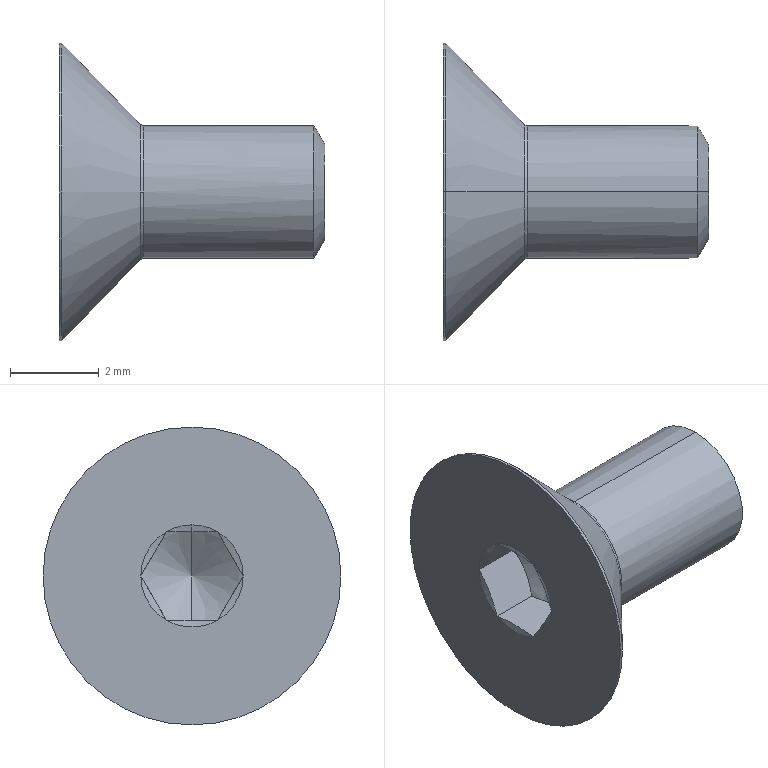Part | SolidWorks | features BaseBody 1 | 1 solid | 27 faces | box 6 x 6.72 x 6.72 mm | volume 61.288 mm3 | cone 13 | plane 8 | cylinder 4 | spline 2 | commonest cylinder face diameters 3 x2 6.72 x2
STEP:
#1=CARTESIAN_POINT('',(-4.169,-1.531,0.));
#2=VERTEX_POINT('',#1);
#3=CARTESIAN_POINT('',(-4.169,0.,1.531));
#4=VERTEX_POINT('',#3);
#5=CARTESIAN_POINT('',(-4.169,0.,0.));
#6=DIRECTION('',(-1.,0.,0.));
#7=DIRECTION('',(0.,-1.,0.));
#8=AXIS2_PLACEMENT_3D('',#5,#6,#7);
#9=CIRCLE('',#8,1.531);
#10=EDGE_CURVE('',#2,#4,#9,.T.);
#11=ORIENTED_EDGE('',*,*,#10,.F.);
#12=CARTESIAN_POINT('',(-4.098,-1.5,0.));
#13=VERTEX_POINT('',#12);
#14=CARTESIAN_POINT('',(-4.098,-1.6,0.));
#15=DIRECTION('',(0.,0.,-1.));
#16=DIRECTION('',(0.,-1.,0.));
#17=AXIS2_PLACEMENT_3D('',#14,#15,#16);
#18=CIRCLE('',#17,0.1);
#19=EDGE_CURVE('',#2,#13,#18,.T.);
#20=ORIENTED_EDGE('',*,*,#19,.T.);
#21=CARTESIAN_POINT('',(-4.098,0.,1.5));
#22=VERTEX_POINT('',#21);
#23=CARTESIAN_POINT('',(-4.098,0.,0.));
#24=DIRECTION('',(1.,0.,0.));
#25=DIRECTION('',(0.,1.,0.));
#26=AXIS2_PLACEMENT_3D('',#23,#24,#25);
#27=CIRCLE('',#26,1.5);
#28=EDGE_CURVE('',#22,#13,#27,.T.);
#29=ORIENTED_EDGE('',*,*,#28,.F.);
#30=CARTESIAN_POINT('',(-4.098,1.5,0.));
#31=VERTEX_POINT('',#30);
#32=CARTESIAN_POINT('',(-4.098,0.,0.));
#33=DIRECTION('',(1.,0.,0.));
#34=DIRECTION('',(0.,1.,0.));
#35=AXIS2_PLACEMENT_3D('',#32,#33,#34);
#36=CIRCLE('',#35,1.5);
#37=EDGE_CURVE('',#31,#22,#36,.T.);
#38=ORIENTED_EDGE('',*,*,#37,.F.);
#39=CARTESIAN_POINT('',(-4.169,1.531,0.));
#40=VERTEX_POINT('',#39);
#41=CARTESIAN_POINT('',(-4.098,1.6,0.));
#42=DIRECTION('',(0.,0.,1.));
#43=DIRECTION('',(0.,1.,0.));
#44=AXIS2_PLACEMENT_3D('',#41,#42,#43);
#45=CIRCLE('',#44,0.1);
#46=EDGE_CURVE('',#40,#31,#45,.T.);
#47=ORIENTED_EDGE('',*,*,#46,.F.);
#48=CARTESIAN_POINT('',(-4.169,0.,0.));
#49=DIRECTION('',(-1.,0.,0.));
#50=DIRECTION('',(0.,-1.,0.));
#51=AXIS2_PLACEMENT_3D('',#48,#49,#50);
#52=CIRCLE('',#51,1.531);
#53=EDGE_CURVE('',#4,#40,#52,.T.);
#54=ORIENTED_EDGE('',*,*,#53,.F.);
#55=EDGE_LOOP('',(#11,#20,#29,#38,#47,#54));
#56=FACE_OUTER_BOUND('',#55,.T.);
#57=CARTESIAN_POINT('',(-4.169,1.531,0.));
#58=CARTESIAN_POINT('',(-4.169,1.531,3.061));
#59=CARTESIAN_POINT('',(-4.169,-1.531,3.061));
#60=CARTESIAN_POINT('',(-4.169,-1.531,0.));
#61=CARTESIAN_POINT('',(-4.15,1.511,0.));
#62=CARTESIAN_POINT('',(-4.15,1.511,3.021));
#63=CARTESIAN_POINT('',(-4.15,-1.511,3.021));
#64=CARTESIAN_POINT('',(-4.15,-1.511,0.));
#65=CARTESIAN_POINT('',(-4.125,1.5,0.));
#66=CARTESIAN_POINT('',(-4.125,1.5,3.));
#67=CARTESIAN_POINT('',(-4.125,-1.5,3.));
#68=CARTESIAN_POINT('',(-4.125,-1.5,0.));
#69=CARTESIAN_POINT('',(-4.098,1.5,0.));
#70=CARTESIAN_POINT('',(-4.098,1.5,3.));
#71=CARTESIAN_POINT('',(-4.098,-1.5,3.));
#72=CARTESIAN_POINT('',(-4.098,-1.5,0.));
#73=(BOUNDED_SURFACE()B_SPLINE_SURFACE(3,3,((#57,#58,#59,#60),(#61,#62,#63,#64),(#65,#66,#67,#68),(#69,#70,#71,#72)),.UNSPECIFIED.,.F.,.F.,.F.)B_SPLINE_SURFACE_WITH_KNOTS((4,4),(4,4),(0.,1.),(0.,1.),.UNSPECIFIED.)GEOMETRIC_REPRESENTATION_ITEM()RATIONAL_B_SPLINE_SURFACE(((1.,0.3333,0.3333,1.),(0.947,0.3157,0.3157,0.947),(0.947,0.3157,0.3157,0.947),(1.,0.3333,0.3333,1.)))REPRESENTATION_ITEM('')SURFACE());
#74=ADVANCED_FACE('',(#56),#73,.F.);
#75=ORIENTED_EDGE('',*,*,#53,.T.);
#76=CARTESIAN_POINT('',(-4.169,0.,-1.531));
#77=VERTEX_POINT('',#76);
#78=CARTESIAN_POINT('',(-4.169,0.,0.));
#79=DIRECTION('',(-1.,0.,0.));
#80=DIRECTION('',(0.,-1.,0.));
#81=AXIS2_PLACEMENT_3D('',#78,#79,#80);
#82=CIRCLE('',#81,1.531);
#83=EDGE_CURVE('',#40,#77,#82,.T.);
#84=ORIENTED_EDGE('',*,*,#83,.T.);
#85=CARTESIAN_POINT('',(-5.936,0.,-3.36));
#86=VERTEX_POINT('',#85);
#87=CARTESIAN_POINT('',(-5.936,0.,-3.36));
#88=DIRECTION('',(-0.6947,0.,-0.7193));
#89=VECTOR('',#88,1000.);
#90=LINE('',#87,#89);
#91=EDGE_CURVE('',#77,#86,#90,.T.);
#92=ORIENTED_EDGE('',*,*,#91,.T.);
#93=CARTESIAN_POINT('',(-5.936,0.,3.36));
#94=VERTEX_POINT('',#93);
#95=CARTESIAN_POINT('',(-5.936,0.,0.));
#96=DIRECTION('',(1.,0.,0.));
#97=DIRECTION('',(0.,-1.,0.));
#98=AXIS2_PLACEMENT_3D('',#95,#96,#97);
#99=CIRCLE('',#98,3.36);
#100=EDGE_CURVE('',#86,#94,#99,.T.);
#101=ORIENTED_EDGE('',*,*,#100,.T.);
#102=CARTESIAN_POINT('',(-5.936,0.,3.36));
#103=DIRECTION('',(-0.6947,0.,0.7193));
#104=VECTOR('',#103,1000.);
#105=LINE('',#102,#104);
#106=EDGE_CURVE('',#4,#94,#105,.T.);
#107=ORIENTED_EDGE('',*,*,#106,.F.);
#108=EDGE_LOOP('',(#75,#84,#92,#101,#107));
#109=FACE_OUTER_BOUND('',#108,.T.);
#110=CARTESIAN_POINT('',(-5.936,0.,0.));
#111=DIRECTION('',(-1.,0.,0.));
#112=DIRECTION('',(0.,0.,1.));
#113=AXIS2_PLACEMENT_3D('',#110,#111,#112);
#114=CONICAL_SURFACE('',#113,3.36,0.8029);
#115=ADVANCED_FACE('',(#109),#114,.T.);
#116=CARTESIAN_POINT('',(-6.,0.,-3.36));
#117=VERTEX_POINT('',#116);
#118=CARTESIAN_POINT('',(-6.,0.,3.36));
#119=VERTEX_POINT('',#118);
#120=CARTESIAN_POINT('',(-6.,0.,0.));
#121=DIRECTION('',(1.,0.,0.));
#122=DIRECTION('',(0.,0.,-1.));
#123=AXIS2_PLACEMENT_3D('',#120,#121,#122);
#124=CIRCLE('',#123,3.36);
#125=EDGE_CURVE('',#117,#119,#124,.T.);
#126=ORIENTED_EDGE('',*,*,#125,.T.);
#127=CARTESIAN_POINT('',(0.,0.,3.36));
#128=DIRECTION('',(1.,0.,0.));
#129=VECTOR('',#128,1000.);
#130=LINE('',#127,#129);
#131=EDGE_CURVE('',#119,#94,#130,.T.);
#132=ORIENTED_EDGE('',*,*,#131,.T.);
#133=ORIENTED_EDGE('',*,*,#100,.F.);
#134=CARTESIAN_POINT('',(0.,0.,-3.36));
#135=DIRECTION('',(1.,0.,0.));
#136=VECTOR('',#135,1000.);
#137=LINE('',#134,#136);
#138=EDGE_CURVE('',#117,#86,#137,.T.);
#139=ORIENTED_EDGE('',*,*,#138,.F.);
#140=EDGE_LOOP('',(#126,#132,#133,#139));
#141=FACE_OUTER_BOUND('',#140,.T.);
#142=CARTESIAN_POINT('',(0.,0.,0.));
#143=DIRECTION('',(1.,0.,0.));
#144=DIRECTION('',(0.,0.,-1.));
#145=AXIS2_PLACEMENT_3D('',#142,#143,#144);
#146=CYLINDRICAL_SURFACE('',#145,3.36);
#147=ADVANCED_FACE('',(#141),#146,.T.);
#148=CARTESIAN_POINT('',(-4.098,0.,-1.5));
#149=VERTEX_POINT('',#148);
#150=CARTESIAN_POINT('',(-4.098,0.,0.));
#151=DIRECTION('',(1.,0.,0.));
#152=DIRECTION('',(0.,1.,0.));
#153=AXIS2_PLACEMENT_3D('',#150,#151,#152);
#154=CIRCLE('',#153,1.5);
#155=EDGE_CURVE('',#149,#31,#154,.T.);
#156=ORIENTED_EDGE('',*,*,#155,.T.);
#157=ORIENTED_EDGE('',*,*,#37,.T.);
#158=CARTESIAN_POINT('',(-0.25,0.,1.5));
#159=VERTEX_POINT('',#158);
#160=CARTESIAN_POINT('',(0.,0.,1.5));
#161=DIRECTION('',(1.,0.,0.));
#162=VECTOR('',#161,1000.);
#163=LINE('',#160,#162);
#164=EDGE_CURVE('',#22,#159,#163,.T.);
#165=ORIENTED_EDGE('',*,*,#164,.T.);
#166=CARTESIAN_POINT('',(-0.25,0.,-1.5));
#167=VERTEX_POINT('',#166);
#168=CARTESIAN_POINT('',(-0.25,0.,0.));
#169=DIRECTION('',(-1.,0.,0.));
#170=DIRECTION('',(0.,0.,-1.));
#171=AXIS2_PLACEMENT_3D('',#168,#169,#170);
#172=CIRCLE('',#171,1.5);
#173=EDGE_CURVE('',#159,#167,#172,.T.);
#174=ORIENTED_EDGE('',*,*,#173,.T.);
#175=CARTESIAN_POINT('',(0.,0.,-1.5));
#176=DIRECTION('',(1.,0.,0.));
#177=VECTOR('',#176,1000.);
#178=LINE('',#175,#177);
#179=EDGE_CURVE('',#149,#167,#178,.T.);
#180=ORIENTED_EDGE('',*,*,#179,.F.);
#181=EDGE_LOOP('',(#156,#157,#165,#174,#180));
#182=FACE_OUTER_BOUND('',#181,.T.);
#183=CARTESIAN_POINT('',(0.,0.,0.));
#184=DIRECTION('',(1.,0.,0.));
#185=DIRECTION('',(0.,0.,-1.));
#186=AXIS2_PLACEMENT_3D('',#183,#184,#185);
#187=CYLINDRICAL_SURFACE('',#186,1.5);
#188=ADVANCED_FACE('',(#182),#187,.T.);
#189=CARTESIAN_POINT('',(0.,0.,1.067));
#190=VERTEX_POINT('',#189);
#191=CARTESIAN_POINT('',(0.,0.,-1.067));
#192=VERTEX_POINT('',#191);
#193=CARTESIAN_POINT('',(0.,0.,0.));
#194=DIRECTION('',(-1.,0.,0.));
#195=DIRECTION('',(0.,0.,1.));
#196=AXIS2_PLACEMENT_3D('',#193,#194,#195);
#197=CIRCLE('',#196,1.067);
#198=EDGE_CURVE('',#190,#192,#197,.T.);
#199=ORIENTED_EDGE('',*,*,#198,.T.);
#200=CARTESIAN_POINT('',(-0.25,0.,-1.5));
#201=DIRECTION('',(-0.5,0.,-0.866));
#202=VECTOR('',#201,1000.);
#203=LINE('',#200,#202);
#204=EDGE_CURVE('',#192,#167,#203,.T.);
#205=ORIENTED_EDGE('',*,*,#204,.T.);
#206=ORIENTED_EDGE('',*,*,#173,.F.);
#207=CARTESIAN_POINT('',(-0.25,0.,1.5));
#208=DIRECTION('',(-0.5,0.,0.866));
#209=VECTOR('',#208,1000.);
#210=LINE('',#207,#209);
#211=EDGE_CURVE('',#190,#159,#210,.T.);
#212=ORIENTED_EDGE('',*,*,#211,.F.);
#213=EDGE_LOOP('',(#199,#205,#206,#212));
#214=FACE_OUTER_BOUND('',#213,.T.);
#215=CARTESIAN_POINT('',(-0.25,0.,0.));
#216=DIRECTION('',(-1.,0.,0.));
#217=DIRECTION('',(0.,0.,1.));
#218=AXIS2_PLACEMENT_3D('',#215,#216,#217);
#219=CONICAL_SURFACE('',#218,1.5,1.047);
#220=ADVANCED_FACE('',(#214),#219,.T.);
#221=CARTESIAN_POINT('',(-5.956,0.,1.));
#222=VERTEX_POINT('',#221);
#223=CARTESIAN_POINT('',(-6.,0.5774,1.));
#224=VERTEX_POINT('',#223);
#225=CARTESIAN_POINT('',(-5.956,0.,1.));
#226=CARTESIAN_POINT('',(-5.956,0.1925,1.));
#227=CARTESIAN_POINT('',(-5.973,0.3849,1.));
#228=CARTESIAN_POINT('',(-6.,0.5774,1.));
#229=B_SPLINE_CURVE_WITH_KNOTS('',3,(#225,#226,#227,#228),.UNSPECIFIED.,.F.,.F.,(4,4),(0.0005774,0.001155),.UNSPECIFIED.);
#230=EDGE_CURVE('',#222,#224,#229,.T.);
#231=ORIENTED_EDGE('',*,*,#230,.F.);
#232=CARTESIAN_POINT('',(-6.,0.,1.155));
#233=VERTEX_POINT('',#232);
#234=CARTESIAN_POINT('',(-6.,0.,1.155));
#235=DIRECTION('',(-0.2748,0.,0.9615));
#236=VECTOR('',#235,1000.);
#237=LINE('',#234,#236);
#238=EDGE_CURVE('',#222,#233,#237,.T.);
#239=ORIENTED_EDGE('',*,*,#238,.T.);
#240=CARTESIAN_POINT('',(-6.,0.,0.));
#241=DIRECTION('',(1.,0.,0.));
#242=DIRECTION('',(0.,0.,1.));
#243=AXIS2_PLACEMENT_3D('',#240,#241,#242);
#244=CIRCLE('',#243,1.155);
#245=EDGE_CURVE('',#224,#233,#244,.T.);
#246=ORIENTED_EDGE('',*,*,#245,.F.);
#247=EDGE_LOOP('',(#231,#239,#246));
#248=FACE_OUTER_BOUND('',#247,.T.);
#249=CARTESIAN_POINT('',(-6.,0.,0.));
#250=DIRECTION('',(-1.,0.,0.));
#251=DIRECTION('',(0.,0.,1.));
#252=AXIS2_PLACEMENT_3D('',#249,#250,#251);
#253=CONICAL_SURFACE('',#252,1.155,1.292);
#254=ADVANCED_FACE('',(#248),#253,.F.);
#255=CARTESIAN_POINT('',(-4.233,0.,0.));
#256=VERTEX_POINT('',#255);
#257=CARTESIAN_POINT('',(-4.811,0.,1.));
#258=VERTEX_POINT('',#257);
#259=CARTESIAN_POINT('',(-4.904,0.,1.162));
#260=DIRECTION('',(-0.5,0.,0.866));
#261=VECTOR('',#260,1000.);
#262=LINE('',#259,#261);
#263=EDGE_CURVE('',#256,#258,#262,.T.);
#264=ORIENTED_EDGE('',*,*,#263,.F.);
#265=CARTESIAN_POINT('',(-4.811,0.,-1.));
#266=VERTEX_POINT('',#265);
#267=CARTESIAN_POINT('',(-4.904,0.,-1.162));
#268=DIRECTION('',(-0.5,0.,-0.866));
#269=VECTOR('',#268,1000.);
#270=LINE('',#267,#269);
#271=EDGE_CURVE('',#256,#266,#270,.T.);
#272=ORIENTED_EDGE('',*,*,#271,.T.);
#273=CARTESIAN_POINT('',(-4.9,-0.5774,-1.));
#274=VERTEX_POINT('',#273);
#275=CARTESIAN_POINT('',(-4.811,0.,-1.));
#276=CARTESIAN_POINT('',(-4.811,-0.196,-1.));
#277=CARTESIAN_POINT('',(-4.846,-0.3889,-1.));
#278=CARTESIAN_POINT('',(-4.9,-0.5774,-1.));
#279=B_SPLINE_CURVE_WITH_KNOTS('',3,(#275,#276,#277,#278),.UNSPECIFIED.,.F.,.F.,(4,4),(0.0005842,0.001166),.UNSPECIFIED.);
#280=EDGE_CURVE('',#266,#274,#279,.T.);
#281=ORIENTED_EDGE('',*,*,#280,.T.);
#282=CARTESIAN_POINT('',(-4.9,-1.155,0.));
#283=VERTEX_POINT('',#282);
#284=CARTESIAN_POINT('',(-4.9,-0.5774,-1.));
#285=CARTESIAN_POINT('',(-4.846,-0.6716,-0.8367));
#286=CARTESIAN_POINT('',(-4.811,-0.7673,-0.671));
#287=CARTESIAN_POINT('',(-4.811,-0.9636,-0.3309));
#288=CARTESIAN_POINT('',(-4.846,-1.06,-0.1635));
#289=CARTESIAN_POINT('',(-4.9,-1.155,0.));
#290=B_SPLINE_CURVE_WITH_KNOTS('',3,(#284,#285,#286,#287,#288,#289),.UNSPECIFIED.,.F.,.F.,(4,2,4),(0.,0.0005831,0.001166),.UNSPECIFIED.);
#291=EDGE_CURVE('',#274,#283,#290,.T.);
#292=ORIENTED_EDGE('',*,*,#291,.T.);
#293=CARTESIAN_POINT('',(-4.9,-0.5774,1.));
#294=VERTEX_POINT('',#293);
#295=CARTESIAN_POINT('',(-4.9,-1.155,0.));
#296=CARTESIAN_POINT('',(-4.846,-1.06,0.1633));
#297=CARTESIAN_POINT('',(-4.811,-0.9647,0.329));
#298=CARTESIAN_POINT('',(-4.811,-0.7684,0.6691));
#299=CARTESIAN_POINT('',(-4.846,-0.6717,0.8365));
#300=CARTESIAN_POINT('',(-4.9,-0.5774,1.));
#301=B_SPLINE_CURVE_WITH_KNOTS('',3,(#295,#296,#297,#298,#299,#300),.UNSPECIFIED.,.F.,.F.,(4,2,4),(0.,0.0005831,0.001166),.UNSPECIFIED.);
#302=EDGE_CURVE('',#283,#294,#301,.T.);
#303=ORIENTED_EDGE('',*,*,#302,.T.);
#304=CARTESIAN_POINT('',(-4.9,-0.5774,1.));
#305=CARTESIAN_POINT('',(-4.845,-0.3885,1.));
#306=CARTESIAN_POINT('',(-4.811,-0.1967,1.));
#307=CARTESIAN_POINT('',(-4.811,0.,1.));
#308=B_SPLINE_CURVE_WITH_KNOTS('',3,(#304,#305,#306,#307),.UNSPECIFIED.,.F.,.F.,(4,4),(0.,0.0005842),.UNSPECIFIED.);
#309=EDGE_CURVE('',#294,#258,#308,.T.);
#310=ORIENTED_EDGE('',*,*,#309,.T.);
#311=EDGE_LOOP('',(#264,#272,#281,#292,#303,#310));
#312=FACE_OUTER_BOUND('',#311,.T.);
#313=CARTESIAN_POINT('',(-4.904,0.,0.));
#314=DIRECTION('',(-1.,0.,0.));
#315=DIRECTION('',(0.,0.,1.));
#316=AXIS2_PLACEMENT_3D('',#313,#314,#315);
#317=CONICAL_SURFACE('',#316,1.162,1.047);
#318=ADVANCED_FACE('',(#312),#317,.F.);
#319=ORIENTED_EDGE('',*,*,#91,.F.);
#320=CARTESIAN_POINT('',(-4.169,0.,0.));
#321=DIRECTION('',(-1.,0.,0.));
#322=DIRECTION('',(0.,-1.,0.));
#323=AXIS2_PLACEMENT_3D('',#320,#321,#322);
#324=CIRCLE('',#323,1.531);
#325=EDGE_CURVE('',#77,#2,#324,.T.);
#326=ORIENTED_EDGE('',*,*,#325,.T.);
#327=ORIENTED_EDGE('',*,*,#10,.T.);
#328=ORIENTED_EDGE('',*,*,#106,.T.);
#329=CARTESIAN_POINT('',(-5.936,0.,0.));
#330=DIRECTION('',(1.,0.,0.));
#331=DIRECTION('',(0.,-1.,0.));
#332=AXIS2_PLACEMENT_3D('',#329,#330,#331);
#333=CIRCLE('',#332,3.36);
#334=EDGE_CURVE('',#94,#86,#333,.T.);
#335=ORIENTED_EDGE('',*,*,#334,.T.);
#336=EDGE_LOOP('',(#319,#326,#327,#328,#335));
#337=FACE_OUTER_BOUND('',#336,.T.);
#338=CARTESIAN_POINT('',(-5.936,0.,0.));
#339=DIRECTION('',(-1.,0.,0.));
#340=DIRECTION('',(0.,0.,1.));
#341=AXIS2_PLACEMENT_3D('',#338,#339,#340);
#342=CONICAL_SURFACE('',#341,3.36,0.8029);
#343=ADVANCED_FACE('',(#337),#342,.T.);
#344=ORIENTED_EDGE('',*,*,#19,.F.);
#345=ORIENTED_EDGE('',*,*,#325,.F.);
#346=ORIENTED_EDGE('',*,*,#83,.F.);
#347=ORIENTED_EDGE('',*,*,#46,.T.);
#348=ORIENTED_EDGE('',*,*,#155,.F.);
#349=CARTESIAN_POINT('',(-4.098,0.,0.));
#350=DIRECTION('',(1.,0.,0.));
#351=DIRECTION('',(0.,1.,0.));
#352=AXIS2_PLACEMENT_3D('',#349,#350,#351);
#353=CIRCLE('',#352,1.5);
#354=EDGE_CURVE('',#13,#149,#353,.T.);
#355=ORIENTED_EDGE('',*,*,#354,.F.);
#356=EDGE_LOOP('',(#344,#345,#346,#347,#348,#355));
#357=FACE_OUTER_BOUND('',#356,.T.);
#358=CARTESIAN_POINT('',(-4.169,-1.531,0.));
#359=CARTESIAN_POINT('',(-4.169,-1.531,-3.061));
#360=CARTESIAN_POINT('',(-4.169,1.531,-3.061));
#361=CARTESIAN_POINT('',(-4.169,1.531,0.));
#362=CARTESIAN_POINT('',(-4.15,-1.511,0.));
#363=CARTESIAN_POINT('',(-4.15,-1.511,-3.021));
#364=CARTESIAN_POINT('',(-4.15,1.511,-3.021));
#365=CARTESIAN_POINT('',(-4.15,1.511,0.));
#366=CARTESIAN_POINT('',(-4.125,-1.5,0.));
#367=CARTESIAN_POINT('',(-4.125,-1.5,-3.));
#368=CARTESIAN_POINT('',(-4.125,1.5,-3.));
#369=CARTESIAN_POINT('',(-4.125,1.5,0.));
#370=CARTESIAN_POINT('',(-4.098,-1.5,0.));
#371=CARTESIAN_POINT('',(-4.098,-1.5,-3.));
#372=CARTESIAN_POINT('',(-4.098,1.5,-3.));
#373=CARTESIAN_POINT('',(-4.098,1.5,0.));
#374=(BOUNDED_SURFACE()B_SPLINE_SURFACE(3,3,((#358,#359,#360,#361),(#362,#363,#364,#365),(#366,#367,#368,#369),(#370,#371,#372,#373)),.UNSPECIFIED.,.F.,.F.,.F.)B_SPLINE_SURFACE_WITH_KNOTS((4,4),(4,4),(0.,1.),(0.,1.),.UNSPECIFIED.)GEOMETRIC_REPRESENTATION_ITEM()RATIONAL_B_SPLINE_SURFACE(((1.,0.3333,0.3333,1.),(0.947,0.3157,0.3157,0.947),(0.947,0.3157,0.3157,0.947),(1.,0.3333,0.3333,1.)))REPRESENTATION_ITEM('')SURFACE());
#375=ADVANCED_FACE('',(#357),#374,.F.);
#376=ORIENTED_EDGE('',*,*,#131,.F.);
#377=CARTESIAN_POINT('',(-6.,0.,0.));
#378=DIRECTION('',(1.,0.,0.));
#379=DIRECTION('',(0.,0.,-1.));
#380=AXIS2_PLACEMENT_3D('',#377,#378,#379);
#381=CIRCLE('',#380,3.36);
#382=EDGE_CURVE('',#119,#117,#381,.T.);
#383=ORIENTED_EDGE('',*,*,#382,.T.);
#384=ORIENTED_EDGE('',*,*,#138,.T.);
#385=ORIENTED_EDGE('',*,*,#334,.F.);
#386=EDGE_LOOP('',(#376,#383,#384,#385));
#387=FACE_OUTER_BOUND('',#386,.T.);
#388=CARTESIAN_POINT('',(0.,0.,0.));
#389=DIRECTION('',(1.,0.,0.));
#390=DIRECTION('',(0.,0.,-1.));
#391=AXIS2_PLACEMENT_3D('',#388,#389,#390);
#392=CYLINDRICAL_SURFACE('',#391,3.36);
#393=ADVANCED_FACE('',(#387),#392,.T.);
#394=ORIENTED_EDGE('',*,*,#164,.F.);
#395=ORIENTED_EDGE('',*,*,#28,.T.);
#396=ORIENTED_EDGE('',*,*,#354,.T.);
#397=ORIENTED_EDGE('',*,*,#179,.T.);
#398=CARTESIAN_POINT('',(-0.25,0.,0.));
#399=DIRECTION('',(-1.,0.,0.));
#400=DIRECTION('',(0.,0.,-1.));
#401=AXIS2_PLACEMENT_3D('',#398,#399,#400);
#402=CIRCLE('',#401,1.5);
#403=EDGE_CURVE('',#167,#159,#402,.T.);
#404=ORIENTED_EDGE('',*,*,#403,.T.);
#405=EDGE_LOOP('',(#394,#395,#396,#397,#404));
#406=FACE_OUTER_BOUND('',#405,.T.);
#407=CARTESIAN_POINT('',(0.,0.,0.));
#408=DIRECTION('',(1.,0.,0.));
#409=DIRECTION('',(0.,0.,-1.));
#410=AXIS2_PLACEMENT_3D('',#407,#408,#409);
#411=CYLINDRICAL_SURFACE('',#410,1.5);
#412=ADVANCED_FACE('',(#406),#411,.T.);
#413=CARTESIAN_POINT('',(-6.,1.155,0.));
#414=VERTEX_POINT('',#413);
#415=CARTESIAN_POINT('',(-6.,0.,0.));
#416=DIRECTION('',(1.,0.,0.));
#417=DIRECTION('',(0.,0.,1.));
#418=AXIS2_PLACEMENT_3D('',#415,#416,#417);
#419=CIRCLE('',#418,1.155);
#420=EDGE_CURVE('',#414,#224,#419,.T.);
#421=ORIENTED_EDGE('',*,*,#420,.T.);
#422=ORIENTED_EDGE('',*,*,#245,.T.);
#423=CARTESIAN_POINT('',(-6.,-0.5774,1.));
#424=VERTEX_POINT('',#423);
#425=CARTESIAN_POINT('',(-6.,0.,0.));
#426=DIRECTION('',(1.,0.,0.));
#427=DIRECTION('',(0.,0.,1.));
#428=AXIS2_PLACEMENT_3D('',#425,#426,#427);
#429=CIRCLE('',#428,1.155);
#430=EDGE_CURVE('',#233,#424,#429,.T.);
#431=ORIENTED_EDGE('',*,*,#430,.T.);
#432=CARTESIAN_POINT('',(-6.,-1.155,0.));
#433=VERTEX_POINT('',#432);
#434=CARTESIAN_POINT('',(-6.,0.,0.));
#435=DIRECTION('',(1.,0.,0.));
#436=DIRECTION('',(0.,0.,1.));
#437=AXIS2_PLACEMENT_3D('',#434,#435,#436);
#438=CIRCLE('',#437,1.155);
#439=EDGE_CURVE('',#424,#433,#438,.T.);
#440=ORIENTED_EDGE('',*,*,#439,.T.);
#441=CARTESIAN_POINT('',(-6.,-0.5774,-1.));
#442=VERTEX_POINT('',#441);
#443=CARTESIAN_POINT('',(-6.,0.,0.));
#444=DIRECTION('',(1.,0.,0.));
#445=DIRECTION('',(0.,0.,1.));
#446=AXIS2_PLACEMENT_3D('',#443,#444,#445);
#447=CIRCLE('',#446,1.155);
#448=EDGE_CURVE('',#433,#442,#447,.T.);
#449=ORIENTED_EDGE('',*,*,#448,.T.);
#450=CARTESIAN_POINT('',(-6.,0.5774,-1.));
#451=VERTEX_POINT('',#450);
#452=CARTESIAN_POINT('',(-6.,0.,0.));
#453=DIRECTION('',(1.,0.,0.));
#454=DIRECTION('',(0.,0.,1.));
#455=AXIS2_PLACEMENT_3D('',#452,#453,#454);
#456=CIRCLE('',#455,1.155);
#457=EDGE_CURVE('',#442,#451,#456,.T.);
#458=ORIENTED_EDGE('',*,*,#457,.T.);
#459=CARTESIAN_POINT('',(-6.,0.,0.));
#460=DIRECTION('',(1.,0.,0.));
#461=DIRECTION('',(0.,0.,1.));
#462=AXIS2_PLACEMENT_3D('',#459,#460,#461);
#463=CIRCLE('',#462,1.155);
#464=EDGE_CURVE('',#451,#414,#463,.T.);
#465=ORIENTED_EDGE('',*,*,#464,.T.);
#466=EDGE_LOOP('',(#421,#422,#431,#440,#449,#458,#465));
#467=FACE_BOUND('',#466,.T.);
#468=ORIENTED_EDGE('',*,*,#125,.F.);
#469=ORIENTED_EDGE('',*,*,#382,.F.);
#470=EDGE_LOOP('',(#468,#469));
#471=FACE_OUTER_BOUND('',#470,.T.);
#472=CARTESIAN_POINT('',(-6.,3.36,0.));
#473=DIRECTION('',(-1.,0.,0.));
#474=DIRECTION('',(0.,0.,1.));
#475=AXIS2_PLACEMENT_3D('',#472,#473,#474);
#476=PLANE('',#475);
#477=ADVANCED_FACE('',(#467,#471),#476,.T.);
#478=ORIENTED_EDGE('',*,*,#204,.F.);
#479=CARTESIAN_POINT('',(0.,0.,0.));
#480=DIRECTION('',(-1.,0.,0.));
#481=DIRECTION('',(0.,0.,1.));
#482=AXIS2_PLACEMENT_3D('',#479,#480,#481);
#483=CIRCLE('',#482,1.067);
#484=EDGE_CURVE('',#192,#190,#483,.T.);
#485=ORIENTED_EDGE('',*,*,#484,.T.);
#486=ORIENTED_EDGE('',*,*,#211,.T.);
#487=ORIENTED_EDGE('',*,*,#403,.F.);
#488=EDGE_LOOP('',(#478,#485,#486,#487));
#489=FACE_OUTER_BOUND('',#488,.T.);
#490=CARTESIAN_POINT('',(-0.25,0.,0.));
#491=DIRECTION('',(-1.,0.,0.));
#492=DIRECTION('',(0.,0.,1.));
#493=AXIS2_PLACEMENT_3D('',#490,#491,#492);
#494=CONICAL_SURFACE('',#493,1.5,1.047);
#495=ADVANCED_FACE('',(#489),#494,.T.);
#496=ORIENTED_EDGE('',*,*,#238,.F.);
#497=CARTESIAN_POINT('',(-6.,-0.5774,1.));
#498=CARTESIAN_POINT('',(-5.973,-0.3849,1.));
#499=CARTESIAN_POINT('',(-5.956,-0.1925,1.));
#500=CARTESIAN_POINT('',(-5.956,0.,1.));
#501=B_SPLINE_CURVE_WITH_KNOTS('',3,(#497,#498,#499,#500),.UNSPECIFIED.,.F.,.F.,(4,4),(0.,0.0005774),.UNSPECIFIED.);
#502=EDGE_CURVE('',#424,#222,#501,.T.);
#503=ORIENTED_EDGE('',*,*,#502,.F.);
#504=ORIENTED_EDGE('',*,*,#430,.F.);
#505=EDGE_LOOP('',(#496,#503,#504));
#506=FACE_OUTER_BOUND('',#505,.T.);
#507=CARTESIAN_POINT('',(-6.,0.,0.));
#508=DIRECTION('',(-1.,0.,0.));
#509=DIRECTION('',(0.,0.,1.));
#510=AXIS2_PLACEMENT_3D('',#507,#508,#509);
#511=CONICAL_SURFACE('',#510,1.155,1.292);
#512=ADVANCED_FACE('',(#506),#511,.F.);
#513=ORIENTED_EDGE('',*,*,#420,.F.);
#514=CARTESIAN_POINT('',(-6.,0.5774,1.));
#515=CARTESIAN_POINT('',(-5.973,0.6736,0.8333));
#516=CARTESIAN_POINT('',(-5.939,0.866,0.5));
#517=CARTESIAN_POINT('',(-5.973,1.058,0.1667));
#518=CARTESIAN_POINT('',(-6.,1.155,0.));
#519=B_SPLINE_CURVE_WITH_KNOTS('',3,(#514,#515,#516,#517,#518),.UNSPECIFIED.,.F.,.F.,(4,1,4),(0.,0.0005774,0.001155),.UNSPECIFIED.);
#520=EDGE_CURVE('',#224,#414,#519,.T.);
#521=ORIENTED_EDGE('',*,*,#520,.F.);
#522=EDGE_LOOP('',(#513,#521));
#523=FACE_OUTER_BOUND('',#522,.T.);
#524=CARTESIAN_POINT('',(-6.,0.,0.));
#525=DIRECTION('',(-1.,0.,0.));
#526=DIRECTION('',(0.,0.,1.));
#527=AXIS2_PLACEMENT_3D('',#524,#525,#526);
#528=CONICAL_SURFACE('',#527,1.155,1.292);
#529=ADVANCED_FACE('',(#523),#528,.F.);
#530=ORIENTED_EDGE('',*,*,#464,.F.);
#531=CARTESIAN_POINT('',(-6.,1.155,0.));
#532=CARTESIAN_POINT('',(-5.973,1.058,-0.1667));
#533=CARTESIAN_POINT('',(-5.939,0.866,-0.5));
#534=CARTESIAN_POINT('',(-5.973,0.6736,-0.8333));
#535=CARTESIAN_POINT('',(-6.,0.5774,-1.));
#536=B_SPLINE_CURVE_WITH_KNOTS('',3,(#531,#532,#533,#534,#535),.UNSPECIFIED.,.F.,.F.,(4,1,4),(0.,0.0005774,0.001155),.UNSPECIFIED.);
#537=EDGE_CURVE('',#414,#451,#536,.T.);
#538=ORIENTED_EDGE('',*,*,#537,.F.);
#539=EDGE_LOOP('',(#530,#538));
#540=FACE_OUTER_BOUND('',#539,.T.);
#541=CARTESIAN_POINT('',(-6.,0.,0.));
#542=DIRECTION('',(-1.,0.,0.));
#543=DIRECTION('',(0.,0.,1.));
#544=AXIS2_PLACEMENT_3D('',#541,#542,#543);
#545=CONICAL_SURFACE('',#544,1.155,1.292);
#546=ADVANCED_FACE('',(#540),#545,.F.);
#547=ORIENTED_EDGE('',*,*,#457,.F.);
#548=CARTESIAN_POINT('',(-6.,0.5774,-1.));
#549=CARTESIAN_POINT('',(-5.973,0.3849,-1.));
#550=CARTESIAN_POINT('',(-5.939,0.,-1.));
#551=CARTESIAN_POINT('',(-5.973,-0.3849,-1.));
#552=CARTESIAN_POINT('',(-6.,-0.5774,-1.));
#553=B_SPLINE_CURVE_WITH_KNOTS('',3,(#548,#549,#550,#551,#552),.UNSPECIFIED.,.F.,.F.,(4,1,4),(0.,0.0005774,0.001155),.UNSPECIFIED.);
#554=EDGE_CURVE('',#451,#442,#553,.T.);
#555=ORIENTED_EDGE('',*,*,#554,.F.);
#556=EDGE_LOOP('',(#547,#555));
#557=FACE_OUTER_BOUND('',#556,.T.);
#558=CARTESIAN_POINT('',(-6.,0.,0.));
#559=DIRECTION('',(-1.,0.,0.));
#560=DIRECTION('',(0.,0.,1.));
#561=AXIS2_PLACEMENT_3D('',#558,#559,#560);
#562=CONICAL_SURFACE('',#561,1.155,1.292);
#563=ADVANCED_FACE('',(#557),#562,.F.);
#564=ORIENTED_EDGE('',*,*,#448,.F.);
#565=CARTESIAN_POINT('',(-6.,-0.5774,-1.));
#566=CARTESIAN_POINT('',(-5.973,-0.6736,-0.8333));
#567=CARTESIAN_POINT('',(-5.939,-0.866,-0.5));
#568=CARTESIAN_POINT('',(-5.973,-1.058,-0.1667));
#569=CARTESIAN_POINT('',(-6.,-1.155,0.));
#570=B_SPLINE_CURVE_WITH_KNOTS('',3,(#565,#566,#567,#568,#569),.UNSPECIFIED.,.F.,.F.,(4,1,4),(0.,0.0005774,0.001155),.UNSPECIFIED.);
#571=EDGE_CURVE('',#442,#433,#570,.T.);
#572=ORIENTED_EDGE('',*,*,#571,.F.);
#573=EDGE_LOOP('',(#564,#572));
#574=FACE_OUTER_BOUND('',#573,.T.);
#575=CARTESIAN_POINT('',(-6.,0.,0.));
#576=DIRECTION('',(-1.,0.,0.));
#577=DIRECTION('',(0.,0.,1.));
#578=AXIS2_PLACEMENT_3D('',#575,#576,#577);
#579=CONICAL_SURFACE('',#578,1.155,1.292);
#580=ADVANCED_FACE('',(#574),#579,.F.);
#581=ORIENTED_EDGE('',*,*,#439,.F.);
#582=CARTESIAN_POINT('',(-6.,-1.155,0.));
#583=CARTESIAN_POINT('',(-5.973,-1.058,0.1667));
#584=CARTESIAN_POINT('',(-5.939,-0.866,0.5));
#585=CARTESIAN_POINT('',(-5.973,-0.6736,0.8333));
#586=CARTESIAN_POINT('',(-6.,-0.5774,1.));
#587=B_SPLINE_CURVE_WITH_KNOTS('',3,(#582,#583,#584,#585,#586),.UNSPECIFIED.,.F.,.F.,(4,1,4),(0.,0.0005774,0.001155),.UNSPECIFIED.);
#588=EDGE_CURVE('',#433,#424,#587,.T.);
#589=ORIENTED_EDGE('',*,*,#588,.F.);
#590=EDGE_LOOP('',(#581,#589));
#591=FACE_OUTER_BOUND('',#590,.T.);
#592=CARTESIAN_POINT('',(-6.,0.,0.));
#593=DIRECTION('',(-1.,0.,0.));
#594=DIRECTION('',(0.,0.,1.));
#595=AXIS2_PLACEMENT_3D('',#592,#593,#594);
#596=CONICAL_SURFACE('',#595,1.155,1.292);
#597=ADVANCED_FACE('',(#591),#596,.F.);
#598=ORIENTED_EDGE('',*,*,#198,.F.);
#599=ORIENTED_EDGE('',*,*,#484,.F.);
#600=EDGE_LOOP('',(#598,#599));
#601=FACE_OUTER_BOUND('',#600,.T.);
#602=CARTESIAN_POINT('',(0.,0.,0.));
#603=DIRECTION('',(1.,0.,0.));
#604=DIRECTION('',(0.,0.,-1.));
#605=AXIS2_PLACEMENT_3D('',#602,#603,#604);
#606=PLANE('',#605);
#607=ADVANCED_FACE('',(#601),#606,.T.);
#608=CARTESIAN_POINT('',(-4.9,0.5774,1.));
#609=VERTEX_POINT('',#608);
#610=CARTESIAN_POINT('',(-4.04,0.5774,1.));
#611=DIRECTION('',(-1.,0.,0.));
#612=VECTOR('',#611,1000.);
#613=LINE('',#610,#612);
#614=EDGE_CURVE('',#609,#224,#613,.T.);
#615=ORIENTED_EDGE('',*,*,#614,.F.);
#616=CARTESIAN_POINT('',(-4.811,0.,1.));
#617=CARTESIAN_POINT('',(-4.811,0.196,1.));
#618=CARTESIAN_POINT('',(-4.846,0.3889,1.));
#619=CARTESIAN_POINT('',(-4.9,0.5774,1.));
#620=B_SPLINE_CURVE_WITH_KNOTS('',3,(#616,#617,#618,#619),.UNSPECIFIED.,.F.,.F.,(4,4),(0.0005842,0.001166),.UNSPECIFIED.);
#621=EDGE_CURVE('',#258,#609,#620,.T.);
#622=ORIENTED_EDGE('',*,*,#621,.F.);
#623=ORIENTED_EDGE('',*,*,#309,.F.);
#624=CARTESIAN_POINT('',(-4.04,-0.5774,1.));
#625=DIRECTION('',(1.,0.,0.));
#626=VECTOR('',#625,1000.);
#627=LINE('',#624,#626);
#628=EDGE_CURVE('',#424,#294,#627,.T.);
#629=ORIENTED_EDGE('',*,*,#628,.F.);
#630=ORIENTED_EDGE('',*,*,#502,.T.);
#631=ORIENTED_EDGE('',*,*,#230,.T.);
#632=EDGE_LOOP('',(#615,#622,#623,#629,#630,#631));
#633=FACE_OUTER_BOUND('',#632,.T.);
#634=CARTESIAN_POINT('',(-4.04,-0.5774,1.));
#635=DIRECTION('',(0.,0.,1.));
#636=DIRECTION('',(0.,-1.,0.));
#637=AXIS2_PLACEMENT_3D('',#634,#635,#636);
#638=PLANE('',#637);
#639=ADVANCED_FACE('',(#633),#638,.F.);
#640=CARTESIAN_POINT('',(-4.9,1.155,0.));
#641=VERTEX_POINT('',#640);
#642=CARTESIAN_POINT('',(-4.04,1.155,0.));
#643=DIRECTION('',(-1.,0.,0.));
#644=VECTOR('',#643,1000.);
#645=LINE('',#642,#644);
#646=EDGE_CURVE('',#641,#414,#645,.T.);
#647=ORIENTED_EDGE('',*,*,#646,.F.);
#648=CARTESIAN_POINT('',(-4.9,0.5774,1.));
#649=CARTESIAN_POINT('',(-4.846,0.6716,0.8367));
#650=CARTESIAN_POINT('',(-4.811,0.7673,0.671));
#651=CARTESIAN_POINT('',(-4.811,0.9636,0.3309));
#652=CARTESIAN_POINT('',(-4.846,1.06,0.1635));
#653=CARTESIAN_POINT('',(-4.9,1.155,0.));
#654=B_SPLINE_CURVE_WITH_KNOTS('',3,(#648,#649,#650,#651,#652,#653),.UNSPECIFIED.,.F.,.F.,(4,2,4),(0.,0.0005831,0.001166),.UNSPECIFIED.);
#655=EDGE_CURVE('',#609,#641,#654,.T.);
#656=ORIENTED_EDGE('',*,*,#655,.F.);
#657=ORIENTED_EDGE('',*,*,#614,.T.);
#658=ORIENTED_EDGE('',*,*,#520,.T.);
#659=EDGE_LOOP('',(#647,#656,#657,#658));
#660=FACE_OUTER_BOUND('',#659,.T.);
#661=CARTESIAN_POINT('',(-4.04,0.5774,1.));
#662=DIRECTION('',(0.,0.866,0.5));
#663=DIRECTION('',(0.,-0.5,0.866));
#664=AXIS2_PLACEMENT_3D('',#661,#662,#663);
#665=PLANE('',#664);
#666=ADVANCED_FACE('',(#660),#665,.F.);
#667=CARTESIAN_POINT('',(-4.9,0.5774,-1.));
#668=VERTEX_POINT('',#667);
#669=CARTESIAN_POINT('',(-4.04,0.5774,-1.));
#670=DIRECTION('',(-1.,0.,0.));
#671=VECTOR('',#670,1000.);
#672=LINE('',#669,#671);
#673=EDGE_CURVE('',#668,#451,#672,.T.);
#674=ORIENTED_EDGE('',*,*,#673,.F.);
#675=CARTESIAN_POINT('',(-4.9,1.155,0.));
#676=CARTESIAN_POINT('',(-4.846,1.06,-0.1633));
#677=CARTESIAN_POINT('',(-4.811,0.9647,-0.329));
#678=CARTESIAN_POINT('',(-4.811,0.7684,-0.6691));
#679=CARTESIAN_POINT('',(-4.846,0.6717,-0.8365));
#680=CARTESIAN_POINT('',(-4.9,0.5774,-1.));
#681=B_SPLINE_CURVE_WITH_KNOTS('',3,(#675,#676,#677,#678,#679,#680),.UNSPECIFIED.,.F.,.F.,(4,2,4),(0.,0.0005831,0.001166),.UNSPECIFIED.);
#682=EDGE_CURVE('',#641,#668,#681,.T.);
#683=ORIENTED_EDGE('',*,*,#682,.F.);
#684=ORIENTED_EDGE('',*,*,#646,.T.);
#685=ORIENTED_EDGE('',*,*,#537,.T.);
#686=EDGE_LOOP('',(#674,#683,#684,#685));
#687=FACE_OUTER_BOUND('',#686,.T.);
#688=CARTESIAN_POINT('',(-4.04,1.155,0.));
#689=DIRECTION('',(0.,0.866,-0.5));
#690=DIRECTION('',(0.,0.5,0.866));
#691=AXIS2_PLACEMENT_3D('',#688,#689,#690);
#692=PLANE('',#691);
#693=ADVANCED_FACE('',(#687),#692,.F.);
#694=CARTESIAN_POINT('',(-4.04,-0.5774,-1.));
#695=DIRECTION('',(-1.,0.,0.));
#696=VECTOR('',#695,1000.);
#697=LINE('',#694,#696);
#698=EDGE_CURVE('',#274,#442,#697,.T.);
#699=ORIENTED_EDGE('',*,*,#698,.F.);
#700=ORIENTED_EDGE('',*,*,#280,.F.);
#701=CARTESIAN_POINT('',(-4.9,0.5774,-1.));
#702=CARTESIAN_POINT('',(-4.845,0.3885,-1.));
#703=CARTESIAN_POINT('',(-4.811,0.1967,-1.));
#704=CARTESIAN_POINT('',(-4.811,0.,-1.));
#705=B_SPLINE_CURVE_WITH_KNOTS('',3,(#701,#702,#703,#704),.UNSPECIFIED.,.F.,.F.,(4,4),(0.,0.0005842),.UNSPECIFIED.);
#706=EDGE_CURVE('',#668,#266,#705,.T.);
#707=ORIENTED_EDGE('',*,*,#706,.F.);
#708=ORIENTED_EDGE('',*,*,#673,.T.);
#709=ORIENTED_EDGE('',*,*,#554,.T.);
#710=EDGE_LOOP('',(#699,#700,#707,#708,#709));
#711=FACE_OUTER_BOUND('',#710,.T.);
#712=CARTESIAN_POINT('',(-4.04,0.5774,-1.));
#713=DIRECTION('',(0.,0.,-1.));
#714=DIRECTION('',(0.,1.,0.));
#715=AXIS2_PLACEMENT_3D('',#712,#713,#714);
#716=PLANE('',#715);
#717=ADVANCED_FACE('',(#711),#716,.F.);
#718=CARTESIAN_POINT('',(-4.04,-1.155,0.));
#719=DIRECTION('',(-1.,0.,0.));
#720=VECTOR('',#719,1000.);
#721=LINE('',#718,#720);
#722=EDGE_CURVE('',#283,#433,#721,.T.);
#723=ORIENTED_EDGE('',*,*,#722,.F.);
#724=ORIENTED_EDGE('',*,*,#291,.F.);
#725=ORIENTED_EDGE('',*,*,#698,.T.);
#726=ORIENTED_EDGE('',*,*,#571,.T.);
#727=EDGE_LOOP('',(#723,#724,#725,#726));
#728=FACE_OUTER_BOUND('',#727,.T.);
#729=CARTESIAN_POINT('',(-4.04,-0.5774,-1.));
#730=DIRECTION('',(0.,-0.866,-0.5));
#731=DIRECTION('',(0.,0.5,-0.866));
#732=AXIS2_PLACEMENT_3D('',#729,#730,#731);
#733=PLANE('',#732);
#734=ADVANCED_FACE('',(#728),#733,.F.);
#735=ORIENTED_EDGE('',*,*,#628,.T.);
#736=ORIENTED_EDGE('',*,*,#302,.F.);
#737=ORIENTED_EDGE('',*,*,#722,.T.);
#738=ORIENTED_EDGE('',*,*,#588,.T.);
#739=EDGE_LOOP('',(#735,#736,#737,#738));
#740=FACE_OUTER_BOUND('',#739,.T.);
#741=CARTESIAN_POINT('',(-4.04,-1.155,0.));
#742=DIRECTION('',(0.,-0.866,0.5));
#743=DIRECTION('',(0.,-0.5,-0.866));
#744=AXIS2_PLACEMENT_3D('',#741,#742,#743);
#745=PLANE('',#744);
#746=ADVANCED_FACE('',(#740),#745,.F.);
#747=ORIENTED_EDGE('',*,*,#271,.F.);
#748=ORIENTED_EDGE('',*,*,#263,.T.);
#749=ORIENTED_EDGE('',*,*,#621,.T.);
#750=ORIENTED_EDGE('',*,*,#655,.T.);
#751=ORIENTED_EDGE('',*,*,#682,.T.);
#752=ORIENTED_EDGE('',*,*,#706,.T.);
#753=EDGE_LOOP('',(#747,#748,#749,#750,#751,#752));
#754=FACE_OUTER_BOUND('',#753,.T.);
#755=CARTESIAN_POINT('',(-4.904,0.,0.));
#756=DIRECTION('',(-1.,0.,0.));
#757=DIRECTION('',(0.,0.,1.));
#758=AXIS2_PLACEMENT_3D('',#755,#756,#757);
#759=CONICAL_SURFACE('',#758,1.162,1.047);
#760=ADVANCED_FACE('',(#754),#759,.F.);
#761=CLOSED_SHELL('',(#74,#115,#147,#188,#220,#254,#318,#343,#375,#393,#412,#477,#495,#512,#529,#546,#563,#580,#597,#607,#639,#666,#693,#717,#734,#746,#760));
#762=MANIFOLD_SOLID_BREP('',#761);
#763=CARTESIAN_POINT('',(0.,0.,0.));
#764=DIRECTION('',(0.,0.,1.));
#765=DIRECTION('',(1.,0.,0.));
#766=AXIS2_PLACEMENT_3D('',#763,#764,#765);
#767=(LENGTH_UNIT()NAMED_UNIT(*)SI_UNIT(.MILLI.,.METRE.));
#768=UNCERTAINTY_MEASURE_WITH_UNIT(LENGTH_MEASURE(0.00001),#767,'','');
#769=(NAMED_UNIT(*)PLANE_ANGLE_UNIT()SI_UNIT($,.RADIAN.));
#770=(NAMED_UNIT(*)SI_UNIT($,.STERADIAN.)SOLID_ANGLE_UNIT());
#771=(GEOMETRIC_REPRESENTATION_CONTEXT(3)GLOBAL_UNCERTAINTY_ASSIGNED_CONTEXT((#768))GLOBAL_UNIT_ASSIGNED_CONTEXT((#767,#769,#770))REPRESENTATION_CONTEXT('',''));
#772=ADVANCED_BREP_SHAPE_REPRESENTATION('',(#762,#766),#771);